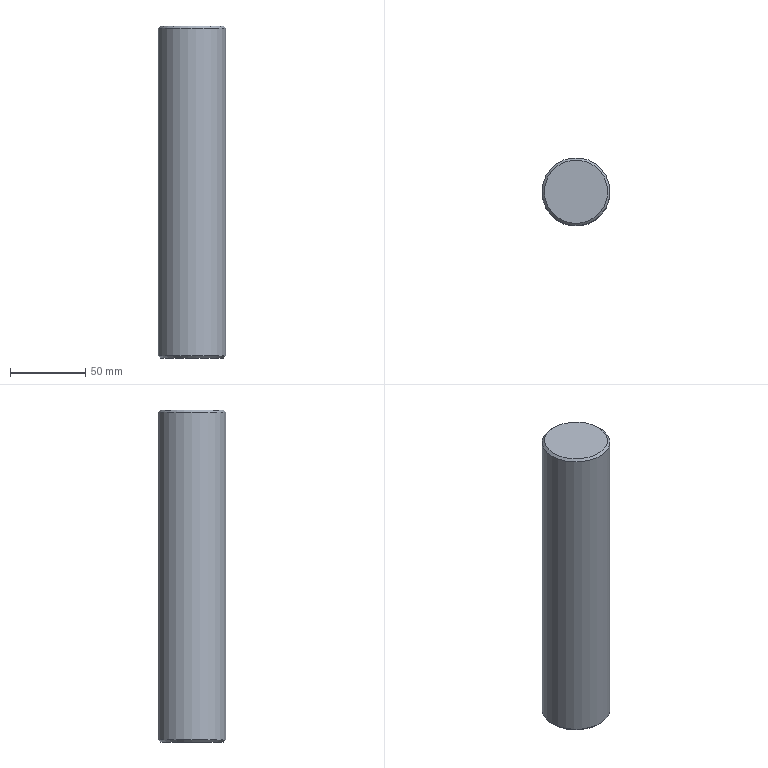Part | STEP file | solid 73 | 1 solid | 9 faces | box 45 x 45 x 220 mm | volume 348635 mm3 | plane 3 | cylinder 3 | cone 3 | commonest cylinder face diameters 6.7 x1 8 x1 45 x1